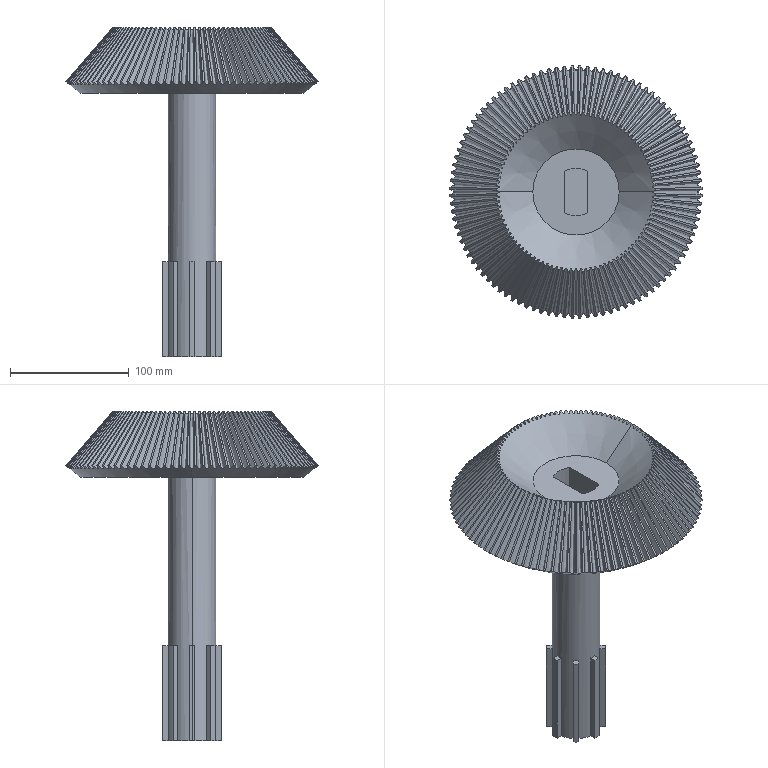Part | SolidWorks | 1 solid | 247 faces | box 211.926 x 211.926 x 276.87 mm | volume 1401987 mm3 | cone 104 | spline 100 | plane 30 | cylinder 13 | commonest cylinder face diameters 50 x9 40 x4